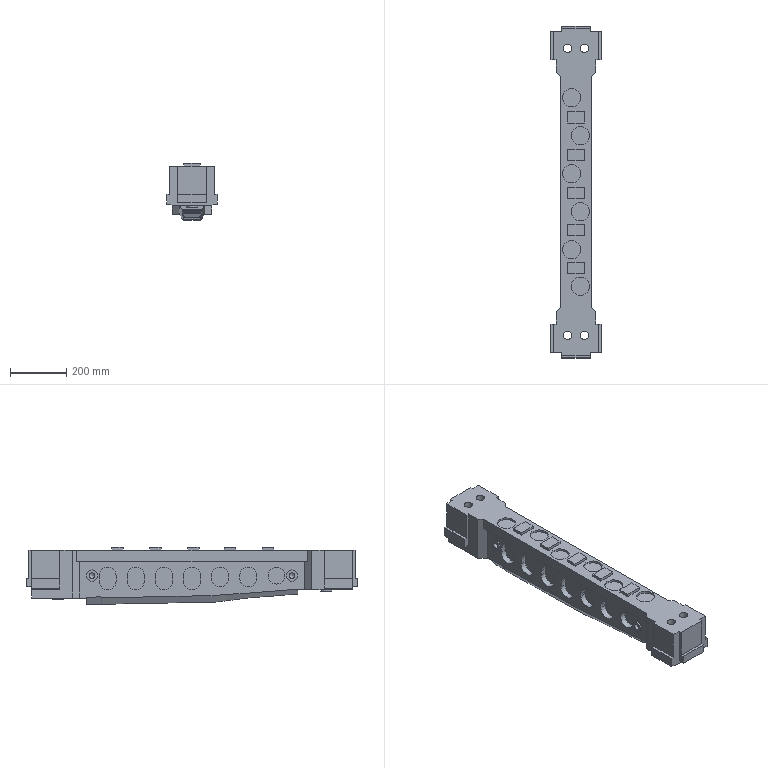Part | NX | features solid 2 | 1 solid | 273 faces | box 180 x 1180 x 202.947 mm | volume 19776894 mm3 | plane 144 | spline 63 | cylinder 58 | cone 6 | sphere 2 | commonest cylinder face diameters 60 x26 20 x6 40 x6 65 x6 10 x4 30 x4